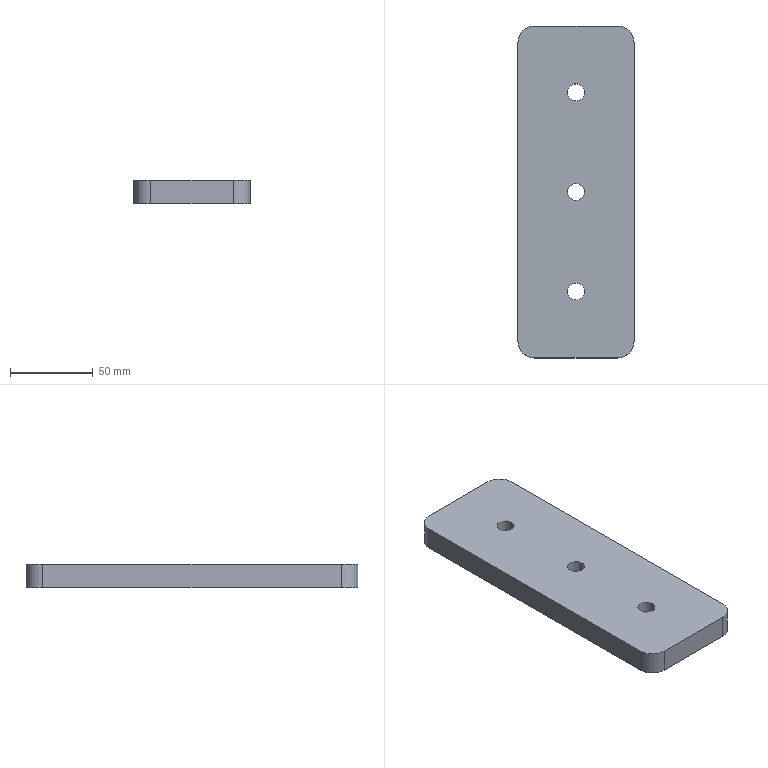Part | SolidWorks | features FlatPattern 1, HoleWzd 1, SMBaseFlange 1, SheetMetal 1 | 1 solid | 16 faces | box 70 x 200 x 14 mm | volume 191366 mm3 | cylinder 10 | plane 6 | commonest cylinder face diameters 10.2 x6 20 x4
STEP:
#1=CARTESIAN_POINT('',(-5.1,0.,-14.));
#2=VERTEX_POINT('',#1);
#3=CARTESIAN_POINT('',(5.1,0.,-14.));
#4=VERTEX_POINT('',#3);
#5=CARTESIAN_POINT('',(0.,0.,-14.));
#6=DIRECTION('',(0.,0.,1.));
#7=DIRECTION('',(1.,0.,0.));
#8=AXIS2_PLACEMENT_3D('',#5,#6,#7);
#9=CIRCLE('',#8,5.1);
#10=EDGE_CURVE('',#2,#4,#9,.T.);
#11=ORIENTED_EDGE('',*,*,#10,.F.);
#12=CARTESIAN_POINT('',(-5.1,0.,0.));
#13=VERTEX_POINT('',#12);
#14=CARTESIAN_POINT('',(-5.1,0.,0.));
#15=DIRECTION('',(0.,0.,1.));
#16=VECTOR('',#15,1000.);
#17=LINE('',#14,#16);
#18=EDGE_CURVE('',#2,#13,#17,.T.);
#19=ORIENTED_EDGE('',*,*,#18,.T.);
#20=CARTESIAN_POINT('',(5.1,0.,0.));
#21=VERTEX_POINT('',#20);
#22=CARTESIAN_POINT('',(0.,0.,0.));
#23=DIRECTION('',(0.,0.,1.));
#24=DIRECTION('',(1.,0.,0.));
#25=AXIS2_PLACEMENT_3D('',#22,#23,#24);
#26=CIRCLE('',#25,5.1);
#27=EDGE_CURVE('',#13,#21,#26,.T.);
#28=ORIENTED_EDGE('',*,*,#27,.T.);
#29=CARTESIAN_POINT('',(5.1,0.,0.));
#30=DIRECTION('',(0.,0.,1.));
#31=VECTOR('',#30,1000.);
#32=LINE('',#29,#31);
#33=EDGE_CURVE('',#4,#21,#32,.T.);
#34=ORIENTED_EDGE('',*,*,#33,.F.);
#35=EDGE_LOOP('',(#11,#19,#28,#34));
#36=FACE_OUTER_BOUND('',#35,.T.);
#37=CARTESIAN_POINT('',(0.,0.,0.));
#38=DIRECTION('',(0.,0.,1.));
#39=DIRECTION('',(1.,0.,0.));
#40=AXIS2_PLACEMENT_3D('',#37,#38,#39);
#41=CYLINDRICAL_SURFACE('',#40,5.1);
#42=ADVANCED_FACE('',(#36),#41,.F.);
#43=CARTESIAN_POINT('',(-5.1,60.,-14.));
#44=VERTEX_POINT('',#43);
#45=CARTESIAN_POINT('',(5.1,60.,-14.));
#46=VERTEX_POINT('',#45);
#47=CARTESIAN_POINT('',(0.,60.,-14.));
#48=DIRECTION('',(0.,0.,1.));
#49=DIRECTION('',(1.,0.,0.));
#50=AXIS2_PLACEMENT_3D('',#47,#48,#49);
#51=CIRCLE('',#50,5.1);
#52=EDGE_CURVE('',#44,#46,#51,.T.);
#53=ORIENTED_EDGE('',*,*,#52,.F.);
#54=CARTESIAN_POINT('',(-5.1,60.,0.));
#55=VERTEX_POINT('',#54);
#56=CARTESIAN_POINT('',(-5.1,60.,0.));
#57=DIRECTION('',(0.,0.,1.));
#58=VECTOR('',#57,1000.);
#59=LINE('',#56,#58);
#60=EDGE_CURVE('',#44,#55,#59,.T.);
#61=ORIENTED_EDGE('',*,*,#60,.T.);
#62=CARTESIAN_POINT('',(5.1,60.,0.));
#63=VERTEX_POINT('',#62);
#64=CARTESIAN_POINT('',(0.,60.,0.));
#65=DIRECTION('',(0.,0.,1.));
#66=DIRECTION('',(1.,0.,0.));
#67=AXIS2_PLACEMENT_3D('',#64,#65,#66);
#68=CIRCLE('',#67,5.1);
#69=EDGE_CURVE('',#55,#63,#68,.T.);
#70=ORIENTED_EDGE('',*,*,#69,.T.);
#71=CARTESIAN_POINT('',(5.1,60.,0.));
#72=DIRECTION('',(0.,0.,1.));
#73=VECTOR('',#72,1000.);
#74=LINE('',#71,#73);
#75=EDGE_CURVE('',#46,#63,#74,.T.);
#76=ORIENTED_EDGE('',*,*,#75,.F.);
#77=EDGE_LOOP('',(#53,#61,#70,#76));
#78=FACE_OUTER_BOUND('',#77,.T.);
#79=CARTESIAN_POINT('',(0.,60.,0.));
#80=DIRECTION('',(0.,0.,1.));
#81=DIRECTION('',(1.,0.,0.));
#82=AXIS2_PLACEMENT_3D('',#79,#80,#81);
#83=CYLINDRICAL_SURFACE('',#82,5.1);
#84=ADVANCED_FACE('',(#78),#83,.F.);
#85=CARTESIAN_POINT('',(-5.1,-60.,-14.));
#86=VERTEX_POINT('',#85);
#87=CARTESIAN_POINT('',(5.1,-60.,-14.));
#88=VERTEX_POINT('',#87);
#89=CARTESIAN_POINT('',(0.,-60.,-14.));
#90=DIRECTION('',(0.,0.,1.));
#91=DIRECTION('',(1.,0.,0.));
#92=AXIS2_PLACEMENT_3D('',#89,#90,#91);
#93=CIRCLE('',#92,5.1);
#94=EDGE_CURVE('',#86,#88,#93,.T.);
#95=ORIENTED_EDGE('',*,*,#94,.F.);
#96=CARTESIAN_POINT('',(-5.1,-60.,0.));
#97=VERTEX_POINT('',#96);
#98=CARTESIAN_POINT('',(-5.1,-60.,0.));
#99=DIRECTION('',(0.,0.,1.));
#100=VECTOR('',#99,1000.);
#101=LINE('',#98,#100);
#102=EDGE_CURVE('',#86,#97,#101,.T.);
#103=ORIENTED_EDGE('',*,*,#102,.T.);
#104=CARTESIAN_POINT('',(5.1,-60.,0.));
#105=VERTEX_POINT('',#104);
#106=CARTESIAN_POINT('',(0.,-60.,0.));
#107=DIRECTION('',(0.,0.,1.));
#108=DIRECTION('',(1.,0.,0.));
#109=AXIS2_PLACEMENT_3D('',#106,#107,#108);
#110=CIRCLE('',#109,5.1);
#111=EDGE_CURVE('',#97,#105,#110,.T.);
#112=ORIENTED_EDGE('',*,*,#111,.T.);
#113=CARTESIAN_POINT('',(5.1,-60.,0.));
#114=DIRECTION('',(0.,0.,1.));
#115=VECTOR('',#114,1000.);
#116=LINE('',#113,#115);
#117=EDGE_CURVE('',#88,#105,#116,.T.);
#118=ORIENTED_EDGE('',*,*,#117,.F.);
#119=EDGE_LOOP('',(#95,#103,#112,#118));
#120=FACE_OUTER_BOUND('',#119,.T.);
#121=CARTESIAN_POINT('',(0.,-60.,0.));
#122=DIRECTION('',(0.,0.,1.));
#123=DIRECTION('',(1.,0.,0.));
#124=AXIS2_PLACEMENT_3D('',#121,#122,#123);
#125=CYLINDRICAL_SURFACE('',#124,5.1);
#126=ADVANCED_FACE('',(#120),#125,.F.);
#127=CARTESIAN_POINT('',(-35.,-90.,0.));
#128=VERTEX_POINT('',#127);
#129=CARTESIAN_POINT('',(-25.,-100.,0.));
#130=VERTEX_POINT('',#129);
#131=CARTESIAN_POINT('',(-25.,-90.,0.));
#132=DIRECTION('',(0.,0.,1.));
#133=DIRECTION('',(1.,0.,0.));
#134=AXIS2_PLACEMENT_3D('',#131,#132,#133);
#135=CIRCLE('',#134,10.);
#136=EDGE_CURVE('',#128,#130,#135,.T.);
#137=ORIENTED_EDGE('',*,*,#136,.F.);
#138=CARTESIAN_POINT('',(-35.,-90.,-14.));
#139=VERTEX_POINT('',#138);
#140=CARTESIAN_POINT('',(-35.,-90.,-14.));
#141=DIRECTION('',(0.,0.,1.));
#142=VECTOR('',#141,1000.);
#143=LINE('',#140,#142);
#144=EDGE_CURVE('',#139,#128,#143,.T.);
#145=ORIENTED_EDGE('',*,*,#144,.F.);
#146=CARTESIAN_POINT('',(-25.,-100.,-14.));
#147=VERTEX_POINT('',#146);
#148=CARTESIAN_POINT('',(-25.,-90.,-14.));
#149=DIRECTION('',(0.,0.,1.));
#150=DIRECTION('',(1.,0.,0.));
#151=AXIS2_PLACEMENT_3D('',#148,#149,#150);
#152=CIRCLE('',#151,10.);
#153=EDGE_CURVE('',#139,#147,#152,.T.);
#154=ORIENTED_EDGE('',*,*,#153,.T.);
#155=CARTESIAN_POINT('',(-25.,-100.,-14.));
#156=DIRECTION('',(0.,0.,1.));
#157=VECTOR('',#156,1000.);
#158=LINE('',#155,#157);
#159=EDGE_CURVE('',#147,#130,#158,.T.);
#160=ORIENTED_EDGE('',*,*,#159,.T.);
#161=EDGE_LOOP('',(#137,#145,#154,#160));
#162=FACE_OUTER_BOUND('',#161,.T.);
#163=CARTESIAN_POINT('',(-25.,-90.,-14.));
#164=DIRECTION('',(0.,0.,1.));
#165=DIRECTION('',(1.,0.,0.));
#166=AXIS2_PLACEMENT_3D('',#163,#164,#165);
#167=CYLINDRICAL_SURFACE('',#166,10.);
#168=ADVANCED_FACE('',(#162),#167,.T.);
#169=CARTESIAN_POINT('',(-35.,90.,0.));
#170=VERTEX_POINT('',#169);
#171=CARTESIAN_POINT('',(-35.,90.,0.));
#172=DIRECTION('',(0.,-1.,0.));
#173=VECTOR('',#172,1000.);
#174=LINE('',#171,#173);
#175=EDGE_CURVE('',#170,#128,#174,.T.);
#176=ORIENTED_EDGE('',*,*,#175,.F.);
#177=CARTESIAN_POINT('',(-35.,90.,-14.));
#178=VERTEX_POINT('',#177);
#179=CARTESIAN_POINT('',(-35.,90.,-14.));
#180=DIRECTION('',(0.,0.,1.));
#181=VECTOR('',#180,1000.);
#182=LINE('',#179,#181);
#183=EDGE_CURVE('',#178,#170,#182,.T.);
#184=ORIENTED_EDGE('',*,*,#183,.F.);
#185=CARTESIAN_POINT('',(-35.,90.,-14.));
#186=DIRECTION('',(0.,-1.,0.));
#187=VECTOR('',#186,1000.);
#188=LINE('',#185,#187);
#189=EDGE_CURVE('',#178,#139,#188,.T.);
#190=ORIENTED_EDGE('',*,*,#189,.T.);
#191=ORIENTED_EDGE('',*,*,#144,.T.);
#192=EDGE_LOOP('',(#176,#184,#190,#191));
#193=FACE_OUTER_BOUND('',#192,.T.);
#194=CARTESIAN_POINT('',(-35.,90.,-14.));
#195=DIRECTION('',(-1.,0.,0.));
#196=DIRECTION('',(0.,-1.,0.));
#197=AXIS2_PLACEMENT_3D('',#194,#195,#196);
#198=PLANE('',#197);
#199=ADVANCED_FACE('',(#193),#198,.T.);
#200=CARTESIAN_POINT('',(-25.,100.,0.));
#201=VERTEX_POINT('',#200);
#202=CARTESIAN_POINT('',(-25.,90.,0.));
#203=DIRECTION('',(0.,0.,1.));
#204=DIRECTION('',(1.,0.,0.));
#205=AXIS2_PLACEMENT_3D('',#202,#203,#204);
#206=CIRCLE('',#205,10.);
#207=EDGE_CURVE('',#201,#170,#206,.T.);
#208=ORIENTED_EDGE('',*,*,#207,.F.);
#209=CARTESIAN_POINT('',(-25.,100.,-14.));
#210=VERTEX_POINT('',#209);
#211=CARTESIAN_POINT('',(-25.,100.,-14.));
#212=DIRECTION('',(0.,0.,1.));
#213=VECTOR('',#212,1000.);
#214=LINE('',#211,#213);
#215=EDGE_CURVE('',#210,#201,#214,.T.);
#216=ORIENTED_EDGE('',*,*,#215,.F.);
#217=CARTESIAN_POINT('',(-25.,90.,-14.));
#218=DIRECTION('',(0.,0.,1.));
#219=DIRECTION('',(1.,0.,0.));
#220=AXIS2_PLACEMENT_3D('',#217,#218,#219);
#221=CIRCLE('',#220,10.);
#222=EDGE_CURVE('',#210,#178,#221,.T.);
#223=ORIENTED_EDGE('',*,*,#222,.T.);
#224=ORIENTED_EDGE('',*,*,#183,.T.);
#225=EDGE_LOOP('',(#208,#216,#223,#224));
#226=FACE_OUTER_BOUND('',#225,.T.);
#227=CARTESIAN_POINT('',(-25.,90.,-14.));
#228=DIRECTION('',(0.,0.,1.));
#229=DIRECTION('',(1.,0.,0.));
#230=AXIS2_PLACEMENT_3D('',#227,#228,#229);
#231=CYLINDRICAL_SURFACE('',#230,10.);
#232=ADVANCED_FACE('',(#226),#231,.T.);
#233=CARTESIAN_POINT('',(25.,100.,0.));
#234=VERTEX_POINT('',#233);
#235=CARTESIAN_POINT('',(-25.,100.,0.));
#236=DIRECTION('',(-1.,0.,0.));
#237=VECTOR('',#236,1000.);
#238=LINE('',#235,#237);
#239=EDGE_CURVE('',#234,#201,#238,.T.);
#240=ORIENTED_EDGE('',*,*,#239,.F.);
#241=CARTESIAN_POINT('',(25.,100.,-14.));
#242=VERTEX_POINT('',#241);
#243=CARTESIAN_POINT('',(25.,100.,-14.));
#244=DIRECTION('',(0.,0.,1.));
#245=VECTOR('',#244,1000.);
#246=LINE('',#243,#245);
#247=EDGE_CURVE('',#242,#234,#246,.T.);
#248=ORIENTED_EDGE('',*,*,#247,.F.);
#249=CARTESIAN_POINT('',(-25.,100.,-14.));
#250=DIRECTION('',(-1.,0.,0.));
#251=VECTOR('',#250,1000.);
#252=LINE('',#249,#251);
#253=EDGE_CURVE('',#242,#210,#252,.T.);
#254=ORIENTED_EDGE('',*,*,#253,.T.);
#255=ORIENTED_EDGE('',*,*,#215,.T.);
#256=EDGE_LOOP('',(#240,#248,#254,#255));
#257=FACE_OUTER_BOUND('',#256,.T.);
#258=CARTESIAN_POINT('',(-25.,100.,-14.));
#259=DIRECTION('',(0.,1.,0.));
#260=DIRECTION('',(0.,0.,1.));
#261=AXIS2_PLACEMENT_3D('',#258,#259,#260);
#262=PLANE('',#261);
#263=ADVANCED_FACE('',(#257),#262,.T.);
#264=CARTESIAN_POINT('',(35.,90.,0.));
#265=VERTEX_POINT('',#264);
#266=CARTESIAN_POINT('',(25.,90.,0.));
#267=DIRECTION('',(0.,0.,1.));
#268=DIRECTION('',(-1.,0.,0.));
#269=AXIS2_PLACEMENT_3D('',#266,#267,#268);
#270=CIRCLE('',#269,10.);
#271=EDGE_CURVE('',#265,#234,#270,.T.);
#272=ORIENTED_EDGE('',*,*,#271,.F.);
#273=CARTESIAN_POINT('',(35.,90.,-14.));
#274=VERTEX_POINT('',#273);
#275=CARTESIAN_POINT('',(35.,90.,-14.));
#276=DIRECTION('',(0.,0.,1.));
#277=VECTOR('',#276,1000.);
#278=LINE('',#275,#277);
#279=EDGE_CURVE('',#274,#265,#278,.T.);
#280=ORIENTED_EDGE('',*,*,#279,.F.);
#281=CARTESIAN_POINT('',(25.,90.,-14.));
#282=DIRECTION('',(0.,0.,1.));
#283=DIRECTION('',(-1.,0.,0.));
#284=AXIS2_PLACEMENT_3D('',#281,#282,#283);
#285=CIRCLE('',#284,10.);
#286=EDGE_CURVE('',#274,#242,#285,.T.);
#287=ORIENTED_EDGE('',*,*,#286,.T.);
#288=ORIENTED_EDGE('',*,*,#247,.T.);
#289=EDGE_LOOP('',(#272,#280,#287,#288));
#290=FACE_OUTER_BOUND('',#289,.T.);
#291=CARTESIAN_POINT('',(25.,90.,-14.));
#292=DIRECTION('',(0.,0.,1.));
#293=DIRECTION('',(1.,0.,0.));
#294=AXIS2_PLACEMENT_3D('',#291,#292,#293);
#295=CYLINDRICAL_SURFACE('',#294,10.);
#296=ADVANCED_FACE('',(#290),#295,.T.);
#297=CARTESIAN_POINT('',(35.,-90.,0.));
#298=VERTEX_POINT('',#297);
#299=CARTESIAN_POINT('',(35.,90.,0.));
#300=DIRECTION('',(0.,1.,0.));
#301=VECTOR('',#300,1000.);
#302=LINE('',#299,#301);
#303=EDGE_CURVE('',#298,#265,#302,.T.);
#304=ORIENTED_EDGE('',*,*,#303,.F.);
#305=CARTESIAN_POINT('',(35.,-90.,-14.));
#306=VERTEX_POINT('',#305);
#307=CARTESIAN_POINT('',(35.,-90.,-14.));
#308=DIRECTION('',(0.,0.,1.));
#309=VECTOR('',#308,1000.);
#310=LINE('',#307,#309);
#311=EDGE_CURVE('',#306,#298,#310,.T.);
#312=ORIENTED_EDGE('',*,*,#311,.F.);
#313=CARTESIAN_POINT('',(35.,90.,-14.));
#314=DIRECTION('',(0.,1.,0.));
#315=VECTOR('',#314,1000.);
#316=LINE('',#313,#315);
#317=EDGE_CURVE('',#306,#274,#316,.T.);
#318=ORIENTED_EDGE('',*,*,#317,.T.);
#319=ORIENTED_EDGE('',*,*,#279,.T.);
#320=EDGE_LOOP('',(#304,#312,#318,#319));
#321=FACE_OUTER_BOUND('',#320,.T.);
#322=CARTESIAN_POINT('',(35.,90.,-14.));
#323=DIRECTION('',(1.,0.,0.));
#324=DIRECTION('',(0.,1.,0.));
#325=AXIS2_PLACEMENT_3D('',#322,#323,#324);
#326=PLANE('',#325);
#327=ADVANCED_FACE('',(#321),#326,.T.);
#328=CARTESIAN_POINT('',(25.,-100.,0.));
#329=VERTEX_POINT('',#328);
#330=CARTESIAN_POINT('',(25.,-90.,0.));
#331=DIRECTION('',(0.,0.,1.));
#332=DIRECTION('',(1.,0.,0.));
#333=AXIS2_PLACEMENT_3D('',#330,#331,#332);
#334=CIRCLE('',#333,10.);
#335=EDGE_CURVE('',#329,#298,#334,.T.);
#336=ORIENTED_EDGE('',*,*,#335,.F.);
#337=CARTESIAN_POINT('',(25.,-100.,-14.));
#338=VERTEX_POINT('',#337);
#339=CARTESIAN_POINT('',(25.,-100.,-14.));
#340=DIRECTION('',(0.,0.,1.));
#341=VECTOR('',#340,1000.);
#342=LINE('',#339,#341);
#343=EDGE_CURVE('',#338,#329,#342,.T.);
#344=ORIENTED_EDGE('',*,*,#343,.F.);
#345=CARTESIAN_POINT('',(25.,-90.,-14.));
#346=DIRECTION('',(0.,0.,1.));
#347=DIRECTION('',(1.,0.,0.));
#348=AXIS2_PLACEMENT_3D('',#345,#346,#347);
#349=CIRCLE('',#348,10.);
#350=EDGE_CURVE('',#338,#306,#349,.T.);
#351=ORIENTED_EDGE('',*,*,#350,.T.);
#352=ORIENTED_EDGE('',*,*,#311,.T.);
#353=EDGE_LOOP('',(#336,#344,#351,#352));
#354=FACE_OUTER_BOUND('',#353,.T.);
#355=CARTESIAN_POINT('',(25.,-90.,-14.));
#356=DIRECTION('',(0.,0.,1.));
#357=DIRECTION('',(1.,0.,0.));
#358=AXIS2_PLACEMENT_3D('',#355,#356,#357);
#359=CYLINDRICAL_SURFACE('',#358,10.);
#360=ADVANCED_FACE('',(#354),#359,.T.);
#361=CARTESIAN_POINT('',(-25.,-100.,0.));
#362=DIRECTION('',(1.,0.,0.));
#363=VECTOR('',#362,1000.);
#364=LINE('',#361,#363);
#365=EDGE_CURVE('',#130,#329,#364,.T.);
#366=ORIENTED_EDGE('',*,*,#365,.F.);
#367=ORIENTED_EDGE('',*,*,#159,.F.);
#368=CARTESIAN_POINT('',(-25.,-100.,-14.));
#369=DIRECTION('',(1.,0.,0.));
#370=VECTOR('',#369,1000.);
#371=LINE('',#368,#370);
#372=EDGE_CURVE('',#147,#338,#371,.T.);
#373=ORIENTED_EDGE('',*,*,#372,.T.);
#374=ORIENTED_EDGE('',*,*,#343,.T.);
#375=EDGE_LOOP('',(#366,#367,#373,#374));
#376=FACE_OUTER_BOUND('',#375,.T.);
#377=CARTESIAN_POINT('',(-25.,-100.,-14.));
#378=DIRECTION('',(0.,-1.,0.));
#379=DIRECTION('',(0.,0.,-1.));
#380=AXIS2_PLACEMENT_3D('',#377,#378,#379);
#381=PLANE('',#380);
#382=ADVANCED_FACE('',(#376),#381,.T.);
#383=CARTESIAN_POINT('',(0.,0.,-14.));
#384=DIRECTION('',(0.,0.,1.));
#385=DIRECTION('',(1.,0.,0.));
#386=AXIS2_PLACEMENT_3D('',#383,#384,#385);
#387=CIRCLE('',#386,5.1);
#388=EDGE_CURVE('',#4,#2,#387,.T.);
#389=ORIENTED_EDGE('',*,*,#388,.T.);
#390=ORIENTED_EDGE('',*,*,#10,.T.);
#391=EDGE_LOOP('',(#389,#390));
#392=FACE_BOUND('',#391,.T.);
#393=CARTESIAN_POINT('',(0.,60.,-14.));
#394=DIRECTION('',(0.,0.,1.));
#395=DIRECTION('',(1.,0.,0.));
#396=AXIS2_PLACEMENT_3D('',#393,#394,#395);
#397=CIRCLE('',#396,5.1);
#398=EDGE_CURVE('',#46,#44,#397,.T.);
#399=ORIENTED_EDGE('',*,*,#398,.T.);
#400=ORIENTED_EDGE('',*,*,#52,.T.);
#401=EDGE_LOOP('',(#399,#400));
#402=FACE_BOUND('',#401,.T.);
#403=CARTESIAN_POINT('',(0.,-60.,-14.));
#404=DIRECTION('',(0.,0.,1.));
#405=DIRECTION('',(1.,0.,0.));
#406=AXIS2_PLACEMENT_3D('',#403,#404,#405);
#407=CIRCLE('',#406,5.1);
#408=EDGE_CURVE('',#88,#86,#407,.T.);
#409=ORIENTED_EDGE('',*,*,#408,.T.);
#410=ORIENTED_EDGE('',*,*,#94,.T.);
#411=EDGE_LOOP('',(#409,#410));
#412=FACE_BOUND('',#411,.T.);
#413=ORIENTED_EDGE('',*,*,#153,.F.);
#414=ORIENTED_EDGE('',*,*,#189,.F.);
#415=ORIENTED_EDGE('',*,*,#222,.F.);
#416=ORIENTED_EDGE('',*,*,#253,.F.);
#417=ORIENTED_EDGE('',*,*,#286,.F.);
#418=ORIENTED_EDGE('',*,*,#317,.F.);
#419=ORIENTED_EDGE('',*,*,#350,.F.);
#420=ORIENTED_EDGE('',*,*,#372,.F.);
#421=EDGE_LOOP('',(#413,#414,#415,#416,#417,#418,#419,#420));
#422=FACE_OUTER_BOUND('',#421,.T.);
#423=CARTESIAN_POINT('',(-25.,-90.,-14.));
#424=DIRECTION('',(0.,0.,1.));
#425=DIRECTION('',(1.,0.,0.));
#426=AXIS2_PLACEMENT_3D('',#423,#424,#425);
#427=PLANE('',#426);
#428=ADVANCED_FACE('',(#392,#402,#412,#422),#427,.F.);
#429=CARTESIAN_POINT('',(0.,0.,0.));
#430=DIRECTION('',(0.,0.,1.));
#431=DIRECTION('',(1.,0.,0.));
#432=AXIS2_PLACEMENT_3D('',#429,#430,#431);
#433=CIRCLE('',#432,5.1);
#434=EDGE_CURVE('',#21,#13,#433,.T.);
#435=ORIENTED_EDGE('',*,*,#434,.F.);
#436=ORIENTED_EDGE('',*,*,#27,.F.);
#437=EDGE_LOOP('',(#435,#436));
#438=FACE_BOUND('',#437,.T.);
#439=CARTESIAN_POINT('',(0.,60.,0.));
#440=DIRECTION('',(0.,0.,1.));
#441=DIRECTION('',(1.,0.,0.));
#442=AXIS2_PLACEMENT_3D('',#439,#440,#441);
#443=CIRCLE('',#442,5.1);
#444=EDGE_CURVE('',#63,#55,#443,.T.);
#445=ORIENTED_EDGE('',*,*,#444,.F.);
#446=ORIENTED_EDGE('',*,*,#69,.F.);
#447=EDGE_LOOP('',(#445,#446));
#448=FACE_BOUND('',#447,.T.);
#449=CARTESIAN_POINT('',(0.,-60.,0.));
#450=DIRECTION('',(0.,0.,1.));
#451=DIRECTION('',(1.,0.,0.));
#452=AXIS2_PLACEMENT_3D('',#449,#450,#451);
#453=CIRCLE('',#452,5.1);
#454=EDGE_CURVE('',#105,#97,#453,.T.);
#455=ORIENTED_EDGE('',*,*,#454,.F.);
#456=ORIENTED_EDGE('',*,*,#111,.F.);
#457=EDGE_LOOP('',(#455,#456));
#458=FACE_BOUND('',#457,.T.);
#459=ORIENTED_EDGE('',*,*,#136,.T.);
#460=ORIENTED_EDGE('',*,*,#365,.T.);
#461=ORIENTED_EDGE('',*,*,#335,.T.);
#462=ORIENTED_EDGE('',*,*,#303,.T.);
#463=ORIENTED_EDGE('',*,*,#271,.T.);
#464=ORIENTED_EDGE('',*,*,#239,.T.);
#465=ORIENTED_EDGE('',*,*,#207,.T.);
#466=ORIENTED_EDGE('',*,*,#175,.T.);
#467=EDGE_LOOP('',(#459,#460,#461,#462,#463,#464,#465,#466));
#468=FACE_OUTER_BOUND('',#467,.T.);
#469=CARTESIAN_POINT('',(-25.,-90.,0.));
#470=DIRECTION('',(0.,0.,1.));
#471=DIRECTION('',(1.,0.,0.));
#472=AXIS2_PLACEMENT_3D('',#469,#470,#471);
#473=PLANE('',#472);
#474=ADVANCED_FACE('',(#438,#448,#458,#468),#473,.T.);
#475=ORIENTED_EDGE('',*,*,#102,.F.);
#476=ORIENTED_EDGE('',*,*,#408,.F.);
#477=ORIENTED_EDGE('',*,*,#117,.T.);
#478=ORIENTED_EDGE('',*,*,#454,.T.);
#479=EDGE_LOOP('',(#475,#476,#477,#478));
#480=FACE_OUTER_BOUND('',#479,.T.);
#481=CARTESIAN_POINT('',(0.,-60.,0.));
#482=DIRECTION('',(0.,0.,1.));
#483=DIRECTION('',(1.,0.,0.));
#484=AXIS2_PLACEMENT_3D('',#481,#482,#483);
#485=CYLINDRICAL_SURFACE('',#484,5.1);
#486=ADVANCED_FACE('',(#480),#485,.F.);
#487=ORIENTED_EDGE('',*,*,#60,.F.);
#488=ORIENTED_EDGE('',*,*,#398,.F.);
#489=ORIENTED_EDGE('',*,*,#75,.T.);
#490=ORIENTED_EDGE('',*,*,#444,.T.);
#491=EDGE_LOOP('',(#487,#488,#489,#490));
#492=FACE_OUTER_BOUND('',#491,.T.);
#493=CARTESIAN_POINT('',(0.,60.,0.));
#494=DIRECTION('',(0.,0.,1.));
#495=DIRECTION('',(1.,0.,0.));
#496=AXIS2_PLACEMENT_3D('',#493,#494,#495);
#497=CYLINDRICAL_SURFACE('',#496,5.1);
#498=ADVANCED_FACE('',(#492),#497,.F.);
#499=ORIENTED_EDGE('',*,*,#18,.F.);
#500=ORIENTED_EDGE('',*,*,#388,.F.);
#501=ORIENTED_EDGE('',*,*,#33,.T.);
#502=ORIENTED_EDGE('',*,*,#434,.T.);
#503=EDGE_LOOP('',(#499,#500,#501,#502));
#504=FACE_OUTER_BOUND('',#503,.T.);
#505=CARTESIAN_POINT('',(0.,0.,0.));
#506=DIRECTION('',(0.,0.,1.));
#507=DIRECTION('',(1.,0.,0.));
#508=AXIS2_PLACEMENT_3D('',#505,#506,#507);
#509=CYLINDRICAL_SURFACE('',#508,5.1);
#510=ADVANCED_FACE('',(#504),#509,.F.);
#511=CLOSED_SHELL('',(#42,#84,#126,#168,#199,#232,#263,#296,#327,#360,#382,#428,#474,#486,#498,#510));
#512=MANIFOLD_SOLID_BREP('',#511);
#513=CARTESIAN_POINT('',(0.,0.,0.));
#514=DIRECTION('',(0.,0.,1.));
#515=DIRECTION('',(1.,0.,0.));
#516=AXIS2_PLACEMENT_3D('',#513,#514,#515);
#517=(LENGTH_UNIT()NAMED_UNIT(*)SI_UNIT(.MILLI.,.METRE.));
#518=UNCERTAINTY_MEASURE_WITH_UNIT(LENGTH_MEASURE(0.00001),#517,'','');
#519=(NAMED_UNIT(*)PLANE_ANGLE_UNIT()SI_UNIT($,.RADIAN.));
#520=(NAMED_UNIT(*)SI_UNIT($,.STERADIAN.)SOLID_ANGLE_UNIT());
#521=(GEOMETRIC_REPRESENTATION_CONTEXT(3)GLOBAL_UNCERTAINTY_ASSIGNED_CONTEXT((#518))GLOBAL_UNIT_ASSIGNED_CONTEXT((#517,#519,#520))REPRESENTATION_CONTEXT('',''));
#522=ADVANCED_BREP_SHAPE_REPRESENTATION('',(#512,#516),#521);